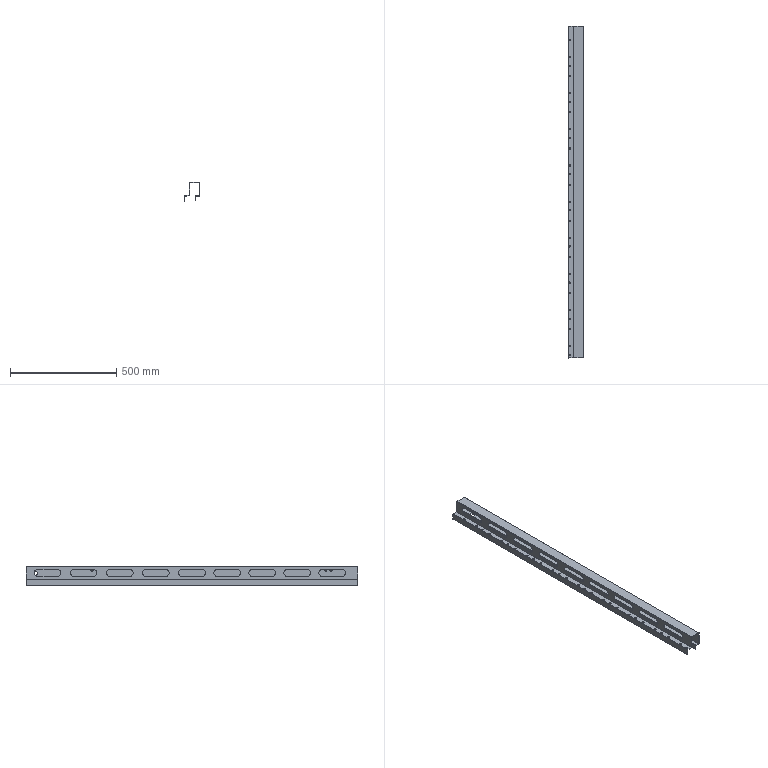Part | SolidWorks | features SplitBody 1 | 1 solid | 362 faces | box 75 x 1562 x 90 mm | volume 568326 mm3 | cylinder 230 | plane 132 | commonest cylinder face diameters 5.5 x66 4.5 x54 9.5 x54 35 x18 6.5 x12 11.5 x12